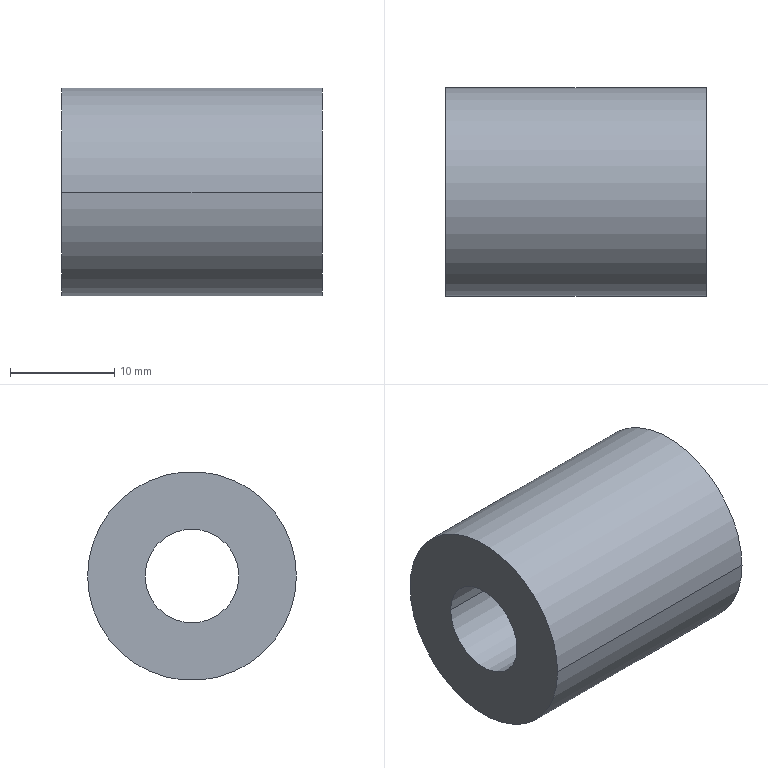Part | STEP file | LM-05-1262 | 1 solid | 6 faces | box 25 x 20 x 20 mm | volume 6264 mm3 | cylinder 4 | plane 2 | commonest cylinder face diameters 9 x2 20 x2
STEP:
#1=CARTESIAN_POINT('',(0.,0.,0.));
#2=DIRECTION('',(0.,0.,1.));
#3=DIRECTION('',(1.,0.,0.));
#4=AXIS2_PLACEMENT_3D('',#1,#2,#3);
#5=CARTESIAN_POINT('',(12.5,-4.5,0.));
#6=VERTEX_POINT('',#5);
#7=CARTESIAN_POINT('',(-12.5,-4.5,0.));
#8=VERTEX_POINT('',#7);
#9=CARTESIAN_POINT('',(12.5,-4.5,0.));
#10=DIRECTION('',(-1.,0.,0.));
#11=VECTOR('',#10,1.);
#12=LINE('',#9,#11);
#13=CARTESIAN_POINT('',(12.5,0.,0.));
#14=DIRECTION('',(-1.,0.,0.));
#15=DIRECTION('',(0.,-1.,0.));
#16=AXIS2_PLACEMENT_3D('',#13,#14,#15);
#17=CYLINDRICAL_SURFACE('',#16,4.5);
#18=CARTESIAN_POINT('',(6.283,0.));
#19=DIRECTION('',(0.,1.));
#20=VECTOR('',#19,1.);
#21=LINE('',#18,#20);
#22=(GEOMETRIC_REPRESENTATION_CONTEXT(2)PARAMETRIC_REPRESENTATION_CONTEXT()REPRESENTATION_CONTEXT('',''));
#23=DEFINITIONAL_REPRESENTATION('',(#21),#22);
#24=PCURVE('',#17,#23);
#25=CARTESIAN_POINT('',(12.5,0.,0.));
#26=DIRECTION('',(-1.,0.,0.));
#27=DIRECTION('',(0.,-1.,0.));
#28=AXIS2_PLACEMENT_3D('',#25,#26,#27);
#29=CYLINDRICAL_SURFACE('',#28,4.5);
#30=CARTESIAN_POINT('',(0.,0.));
#31=DIRECTION('',(0.,1.));
#32=VECTOR('',#31,1.);
#33=LINE('',#30,#32);
#34=(GEOMETRIC_REPRESENTATION_CONTEXT(2)PARAMETRIC_REPRESENTATION_CONTEXT()REPRESENTATION_CONTEXT('',''));
#35=DEFINITIONAL_REPRESENTATION('',(#33),#34);
#36=PCURVE('',#29,#35);
#37=SURFACE_CURVE('',#12,(#24,#36),.PCURVE_S1.);
#38=EDGE_CURVE('',#6,#8,#37,.T.);
#39=ORIENTED_EDGE('',*,*,#38,.T.);
#40=CARTESIAN_POINT('',(-12.5,4.5,0.));
#41=VERTEX_POINT('',#40);
#42=CARTESIAN_POINT('',(-12.5,0.,0.));
#43=DIRECTION('',(-1.,0.,0.));
#44=DIRECTION('',(0.,-1.,0.));
#45=AXIS2_PLACEMENT_3D('',#42,#43,#44);
#46=CIRCLE('',#45,4.5);
#47=CARTESIAN_POINT('',(0.,25.));
#48=DIRECTION('',(1.,0.));
#49=VECTOR('',#48,1.);
#50=LINE('',#47,#49);
#51=(GEOMETRIC_REPRESENTATION_CONTEXT(2)PARAMETRIC_REPRESENTATION_CONTEXT()REPRESENTATION_CONTEXT('',''));
#52=DEFINITIONAL_REPRESENTATION('',(#50),#51);
#53=PCURVE('',#17,#52);
#54=CARTESIAN_POINT('',(-12.5,4.5,0.));
#55=DIRECTION('',(-1.,0.,0.));
#56=DIRECTION('',(0.,-1.,0.));
#57=AXIS2_PLACEMENT_3D('',#54,#55,#56);
#58=PLANE('',#57);
#59=CARTESIAN_POINT('',(4.5,0.));
#60=DIRECTION('',(1.,0.));
#61=AXIS2_PLACEMENT_2D('',#59,#60);
#62=CIRCLE('',#61,4.5);
#63=(GEOMETRIC_REPRESENTATION_CONTEXT(2)PARAMETRIC_REPRESENTATION_CONTEXT()REPRESENTATION_CONTEXT('',''));
#64=DEFINITIONAL_REPRESENTATION('',(#62),#63);
#65=PCURVE('',#58,#64);
#66=SURFACE_CURVE('',#46,(#53,#65),.PCURVE_S1.);
#67=EDGE_CURVE('',#41,#8,#66,.T.);
#68=ORIENTED_EDGE('',*,*,#67,.F.);
#69=CARTESIAN_POINT('',(12.5,4.5,0.));
#70=VERTEX_POINT('',#69);
#71=CARTESIAN_POINT('',(12.5,4.5,0.));
#72=DIRECTION('',(-1.,0.,0.));
#73=VECTOR('',#72,1.);
#74=LINE('',#71,#73);
#75=CARTESIAN_POINT('',(3.142,0.));
#76=DIRECTION('',(0.,1.));
#77=VECTOR('',#76,1.);
#78=LINE('',#75,#77);
#79=(GEOMETRIC_REPRESENTATION_CONTEXT(2)PARAMETRIC_REPRESENTATION_CONTEXT()REPRESENTATION_CONTEXT('',''));
#80=DEFINITIONAL_REPRESENTATION('',(#78),#79);
#81=PCURVE('',#17,#80);
#82=CARTESIAN_POINT('',(3.142,0.));
#83=DIRECTION('',(0.,1.));
#84=VECTOR('',#83,1.);
#85=LINE('',#82,#84);
#86=(GEOMETRIC_REPRESENTATION_CONTEXT(2)PARAMETRIC_REPRESENTATION_CONTEXT()REPRESENTATION_CONTEXT('',''));
#87=DEFINITIONAL_REPRESENTATION('',(#85),#86);
#88=PCURVE('',#29,#87);
#89=SURFACE_CURVE('',#74,(#81,#88),.PCURVE_S1.);
#90=EDGE_CURVE('',#70,#41,#89,.T.);
#91=ORIENTED_EDGE('',*,*,#90,.F.);
#92=CARTESIAN_POINT('',(12.5,0.,0.));
#93=DIRECTION('',(-1.,0.,0.));
#94=DIRECTION('',(0.,-1.,0.));
#95=AXIS2_PLACEMENT_3D('',#92,#93,#94);
#96=CIRCLE('',#95,4.5);
#97=CARTESIAN_POINT('',(0.,0.));
#98=DIRECTION('',(1.,0.));
#99=VECTOR('',#98,1.);
#100=LINE('',#97,#99);
#101=(GEOMETRIC_REPRESENTATION_CONTEXT(2)PARAMETRIC_REPRESENTATION_CONTEXT()REPRESENTATION_CONTEXT('',''));
#102=DEFINITIONAL_REPRESENTATION('',(#100),#101);
#103=PCURVE('',#17,#102);
#104=CARTESIAN_POINT('',(12.5,10.,0.));
#105=DIRECTION('',(1.,0.,0.));
#106=DIRECTION('',(0.,1.,0.));
#107=AXIS2_PLACEMENT_3D('',#104,#105,#106);
#108=PLANE('',#107);
#109=CARTESIAN_POINT('',(-14.5,0.));
#110=CARTESIAN_POINT('',(-14.5,7.794));
#111=CARTESIAN_POINT('',(-7.75,3.897));
#112=CARTESIAN_POINT('',(-1.,0.));
#113=CARTESIAN_POINT('',(-7.75,-3.897));
#114=CARTESIAN_POINT('',(-14.5,-7.794));
#115=CARTESIAN_POINT('',(-14.5,0.));
#116=(BOUNDED_CURVE()B_SPLINE_CURVE(2,(#109,#110,#111,#112,#113,#114,#115),.UNSPECIFIED.,.T.,.F.)B_SPLINE_CURVE_WITH_KNOTS((1,2,2,2,2,1),(-2.094,0.,2.094,4.189,6.283,8.378),.UNSPECIFIED.)CURVE()GEOMETRIC_REPRESENTATION_ITEM()RATIONAL_B_SPLINE_CURVE((1.,0.5,1.,0.5,1.,0.5,1.))REPRESENTATION_ITEM(''));
#117=(GEOMETRIC_REPRESENTATION_CONTEXT(2)PARAMETRIC_REPRESENTATION_CONTEXT()REPRESENTATION_CONTEXT('',''));
#118=DEFINITIONAL_REPRESENTATION('',(#116),#117);
#119=PCURVE('',#108,#118);
#120=SURFACE_CURVE('',#96,(#103,#119),.PCURVE_S1.);
#121=EDGE_CURVE('',#70,#6,#120,.T.);
#122=ORIENTED_EDGE('',*,*,#121,.T.);
#123=EDGE_LOOP('',(#39,#68,#91,#122));
#124=FACE_BOUND('',#123,.F.);
#125=ADVANCED_FACE('',(#124),#17,.F.);
#126=CARTESIAN_POINT('',(12.5,-10.,0.));
#127=VERTEX_POINT('',#126);
#128=CARTESIAN_POINT('',(12.5,10.,0.));
#129=VERTEX_POINT('',#128);
#130=CARTESIAN_POINT('',(12.5,0.,0.));
#131=DIRECTION('',(-1.,0.,0.));
#132=DIRECTION('',(0.,-1.,0.));
#133=AXIS2_PLACEMENT_3D('',#130,#131,#132);
#134=CIRCLE('',#133,10.);
#135=CARTESIAN_POINT('',(12.5,0.,0.));
#136=DIRECTION('',(-1.,0.,0.));
#137=DIRECTION('',(0.,-1.,0.));
#138=AXIS2_PLACEMENT_3D('',#135,#136,#137);
#139=CYLINDRICAL_SURFACE('',#138,10.);
#140=CARTESIAN_POINT('',(0.,0.));
#141=DIRECTION('',(1.,0.));
#142=VECTOR('',#141,1.);
#143=LINE('',#140,#142);
#144=(GEOMETRIC_REPRESENTATION_CONTEXT(2)PARAMETRIC_REPRESENTATION_CONTEXT()REPRESENTATION_CONTEXT('',''));
#145=DEFINITIONAL_REPRESENTATION('',(#143),#144);
#146=PCURVE('',#139,#145);
#147=CARTESIAN_POINT('',(-20.,0.));
#148=CARTESIAN_POINT('',(-20.,17.321));
#149=CARTESIAN_POINT('',(-5.,8.66));
#150=CARTESIAN_POINT('',(10.,0.));
#151=CARTESIAN_POINT('',(-5.,-8.66));
#152=CARTESIAN_POINT('',(-20.,-17.321));
#153=CARTESIAN_POINT('',(-20.,0.));
#154=(BOUNDED_CURVE()B_SPLINE_CURVE(2,(#147,#148,#149,#150,#151,#152,#153),.UNSPECIFIED.,.T.,.F.)B_SPLINE_CURVE_WITH_KNOTS((1,2,2,2,2,1),(-2.094,0.,2.094,4.189,6.283,8.378),.UNSPECIFIED.)CURVE()GEOMETRIC_REPRESENTATION_ITEM()RATIONAL_B_SPLINE_CURVE((1.,0.5,1.,0.5,1.,0.5,1.))REPRESENTATION_ITEM(''));
#155=(GEOMETRIC_REPRESENTATION_CONTEXT(2)PARAMETRIC_REPRESENTATION_CONTEXT()REPRESENTATION_CONTEXT('',''));
#156=DEFINITIONAL_REPRESENTATION('',(#154),#155);
#157=PCURVE('',#108,#156);
#158=SURFACE_CURVE('',#134,(#146,#157),.PCURVE_S1.);
#159=EDGE_CURVE('',#127,#129,#158,.T.);
#160=ORIENTED_EDGE('',*,*,#159,.T.);
#161=CARTESIAN_POINT('',(-12.5,10.,0.));
#162=VERTEX_POINT('',#161);
#163=CARTESIAN_POINT('',(12.5,10.,0.));
#164=DIRECTION('',(-1.,0.,0.));
#165=VECTOR('',#164,1.);
#166=LINE('',#163,#165);
#167=CARTESIAN_POINT('',(3.142,0.));
#168=DIRECTION('',(0.,1.));
#169=VECTOR('',#168,1.);
#170=LINE('',#167,#169);
#171=(GEOMETRIC_REPRESENTATION_CONTEXT(2)PARAMETRIC_REPRESENTATION_CONTEXT()REPRESENTATION_CONTEXT('',''));
#172=DEFINITIONAL_REPRESENTATION('',(#170),#171);
#173=PCURVE('',#139,#172);
#174=CARTESIAN_POINT('',(12.5,0.,0.));
#175=DIRECTION('',(-1.,0.,0.));
#176=DIRECTION('',(0.,-1.,0.));
#177=AXIS2_PLACEMENT_3D('',#174,#175,#176);
#178=CYLINDRICAL_SURFACE('',#177,10.);
#179=CARTESIAN_POINT('',(3.142,0.));
#180=DIRECTION('',(0.,1.));
#181=VECTOR('',#180,1.);
#182=LINE('',#179,#181);
#183=(GEOMETRIC_REPRESENTATION_CONTEXT(2)PARAMETRIC_REPRESENTATION_CONTEXT()REPRESENTATION_CONTEXT('',''));
#184=DEFINITIONAL_REPRESENTATION('',(#182),#183);
#185=PCURVE('',#178,#184);
#186=SURFACE_CURVE('',#166,(#173,#185),.PCURVE_S1.);
#187=EDGE_CURVE('',#129,#162,#186,.T.);
#188=ORIENTED_EDGE('',*,*,#187,.T.);
#189=CARTESIAN_POINT('',(-12.5,-10.,0.));
#190=VERTEX_POINT('',#189);
#191=CARTESIAN_POINT('',(-12.5,0.,0.));
#192=DIRECTION('',(-1.,0.,0.));
#193=DIRECTION('',(0.,-1.,0.));
#194=AXIS2_PLACEMENT_3D('',#191,#192,#193);
#195=CIRCLE('',#194,10.);
#196=CARTESIAN_POINT('',(0.,25.));
#197=DIRECTION('',(1.,0.));
#198=VECTOR('',#197,1.);
#199=LINE('',#196,#198);
#200=(GEOMETRIC_REPRESENTATION_CONTEXT(2)PARAMETRIC_REPRESENTATION_CONTEXT()REPRESENTATION_CONTEXT('',''));
#201=DEFINITIONAL_REPRESENTATION('',(#199),#200);
#202=PCURVE('',#139,#201);
#203=CARTESIAN_POINT('',(4.5,0.));
#204=DIRECTION('',(1.,0.));
#205=AXIS2_PLACEMENT_2D('',#203,#204);
#206=CIRCLE('',#205,10.);
#207=(GEOMETRIC_REPRESENTATION_CONTEXT(2)PARAMETRIC_REPRESENTATION_CONTEXT()REPRESENTATION_CONTEXT('',''));
#208=DEFINITIONAL_REPRESENTATION('',(#206),#207);
#209=PCURVE('',#58,#208);
#210=SURFACE_CURVE('',#195,(#202,#209),.PCURVE_S1.);
#211=EDGE_CURVE('',#190,#162,#210,.T.);
#212=ORIENTED_EDGE('',*,*,#211,.F.);
#213=CARTESIAN_POINT('',(12.5,-10.,0.));
#214=DIRECTION('',(-1.,0.,0.));
#215=VECTOR('',#214,1.);
#216=LINE('',#213,#215);
#217=CARTESIAN_POINT('',(0.,0.));
#218=DIRECTION('',(0.,1.));
#219=VECTOR('',#218,1.);
#220=LINE('',#217,#219);
#221=(GEOMETRIC_REPRESENTATION_CONTEXT(2)PARAMETRIC_REPRESENTATION_CONTEXT()REPRESENTATION_CONTEXT('',''));
#222=DEFINITIONAL_REPRESENTATION('',(#220),#221);
#223=PCURVE('',#139,#222);
#224=CARTESIAN_POINT('',(6.283,0.));
#225=DIRECTION('',(0.,1.));
#226=VECTOR('',#225,1.);
#227=LINE('',#224,#226);
#228=(GEOMETRIC_REPRESENTATION_CONTEXT(2)PARAMETRIC_REPRESENTATION_CONTEXT()REPRESENTATION_CONTEXT('',''));
#229=DEFINITIONAL_REPRESENTATION('',(#227),#228);
#230=PCURVE('',#178,#229);
#231=SURFACE_CURVE('',#216,(#223,#230),.PCURVE_S1.);
#232=EDGE_CURVE('',#127,#190,#231,.T.);
#233=ORIENTED_EDGE('',*,*,#232,.F.);
#234=EDGE_LOOP('',(#160,#188,#212,#233));
#235=FACE_BOUND('',#234,.T.);
#236=ADVANCED_FACE('',(#235),#139,.T.);
#237=ORIENTED_EDGE('',*,*,#187,.F.);
#238=CARTESIAN_POINT('',(12.5,0.,0.));
#239=DIRECTION('',(-1.,0.,0.));
#240=DIRECTION('',(0.,-1.,0.));
#241=AXIS2_PLACEMENT_3D('',#238,#239,#240);
#242=CIRCLE('',#241,10.);
#243=CARTESIAN_POINT('',(0.,0.));
#244=DIRECTION('',(1.,0.));
#245=VECTOR('',#244,1.);
#246=LINE('',#243,#245);
#247=(GEOMETRIC_REPRESENTATION_CONTEXT(2)PARAMETRIC_REPRESENTATION_CONTEXT()REPRESENTATION_CONTEXT('',''));
#248=DEFINITIONAL_REPRESENTATION('',(#246),#247);
#249=PCURVE('',#178,#248);
#250=CARTESIAN_POINT('',(-20.,0.));
#251=CARTESIAN_POINT('',(-20.,17.321));
#252=CARTESIAN_POINT('',(-5.,8.66));
#253=CARTESIAN_POINT('',(10.,0.));
#254=CARTESIAN_POINT('',(-5.,-8.66));
#255=CARTESIAN_POINT('',(-20.,-17.321));
#256=CARTESIAN_POINT('',(-20.,0.));
#257=(BOUNDED_CURVE()B_SPLINE_CURVE(2,(#250,#251,#252,#253,#254,#255,#256),.UNSPECIFIED.,.T.,.F.)B_SPLINE_CURVE_WITH_KNOTS((1,2,2,2,2,1),(-2.094,0.,2.094,4.189,6.283,8.378),.UNSPECIFIED.)CURVE()GEOMETRIC_REPRESENTATION_ITEM()RATIONAL_B_SPLINE_CURVE((1.,0.5,1.,0.5,1.,0.5,1.))REPRESENTATION_ITEM(''));
#258=(GEOMETRIC_REPRESENTATION_CONTEXT(2)PARAMETRIC_REPRESENTATION_CONTEXT()REPRESENTATION_CONTEXT('',''));
#259=DEFINITIONAL_REPRESENTATION('',(#257),#258);
#260=PCURVE('',#108,#259);
#261=SURFACE_CURVE('',#242,(#249,#260),.PCURVE_S1.);
#262=EDGE_CURVE('',#129,#127,#261,.T.);
#263=ORIENTED_EDGE('',*,*,#262,.T.);
#264=ORIENTED_EDGE('',*,*,#232,.T.);
#265=CARTESIAN_POINT('',(-12.5,0.,0.));
#266=DIRECTION('',(-1.,0.,0.));
#267=DIRECTION('',(0.,-1.,0.));
#268=AXIS2_PLACEMENT_3D('',#265,#266,#267);
#269=CIRCLE('',#268,10.);
#270=CARTESIAN_POINT('',(0.,25.));
#271=DIRECTION('',(1.,0.));
#272=VECTOR('',#271,1.);
#273=LINE('',#270,#272);
#274=(GEOMETRIC_REPRESENTATION_CONTEXT(2)PARAMETRIC_REPRESENTATION_CONTEXT()REPRESENTATION_CONTEXT('',''));
#275=DEFINITIONAL_REPRESENTATION('',(#273),#274);
#276=PCURVE('',#178,#275);
#277=CARTESIAN_POINT('',(4.5,0.));
#278=DIRECTION('',(1.,0.));
#279=AXIS2_PLACEMENT_2D('',#277,#278);
#280=CIRCLE('',#279,10.);
#281=(GEOMETRIC_REPRESENTATION_CONTEXT(2)PARAMETRIC_REPRESENTATION_CONTEXT()REPRESENTATION_CONTEXT('',''));
#282=DEFINITIONAL_REPRESENTATION('',(#280),#281);
#283=PCURVE('',#58,#282);
#284=SURFACE_CURVE('',#269,(#276,#283),.PCURVE_S1.);
#285=EDGE_CURVE('',#162,#190,#284,.T.);
#286=ORIENTED_EDGE('',*,*,#285,.F.);
#287=EDGE_LOOP('',(#237,#263,#264,#286));
#288=FACE_BOUND('',#287,.T.);
#289=ADVANCED_FACE('',(#288),#178,.T.);
#290=CARTESIAN_POINT('',(12.5,0.,0.));
#291=DIRECTION('',(-1.,0.,0.));
#292=DIRECTION('',(0.,-1.,0.));
#293=AXIS2_PLACEMENT_3D('',#290,#291,#292);
#294=CIRCLE('',#293,4.5);
#295=CARTESIAN_POINT('',(-14.5,0.));
#296=CARTESIAN_POINT('',(-14.5,7.794));
#297=CARTESIAN_POINT('',(-7.75,3.897));
#298=CARTESIAN_POINT('',(-1.,0.));
#299=CARTESIAN_POINT('',(-7.75,-3.897));
#300=CARTESIAN_POINT('',(-14.5,-7.794));
#301=CARTESIAN_POINT('',(-14.5,0.));
#302=(BOUNDED_CURVE()B_SPLINE_CURVE(2,(#295,#296,#297,#298,#299,#300,#301),.UNSPECIFIED.,.T.,.F.)B_SPLINE_CURVE_WITH_KNOTS((1,2,2,2,2,1),(-2.094,0.,2.094,4.189,6.283,8.378),.UNSPECIFIED.)CURVE()GEOMETRIC_REPRESENTATION_ITEM()RATIONAL_B_SPLINE_CURVE((1.,0.5,1.,0.5,1.,0.5,1.))REPRESENTATION_ITEM(''));
#303=(GEOMETRIC_REPRESENTATION_CONTEXT(2)PARAMETRIC_REPRESENTATION_CONTEXT()REPRESENTATION_CONTEXT('',''));
#304=DEFINITIONAL_REPRESENTATION('',(#302),#303);
#305=PCURVE('',#108,#304);
#306=CARTESIAN_POINT('',(0.,0.));
#307=DIRECTION('',(1.,0.));
#308=VECTOR('',#307,1.);
#309=LINE('',#306,#308);
#310=(GEOMETRIC_REPRESENTATION_CONTEXT(2)PARAMETRIC_REPRESENTATION_CONTEXT()REPRESENTATION_CONTEXT('',''));
#311=DEFINITIONAL_REPRESENTATION('',(#309),#310);
#312=PCURVE('',#29,#311);
#313=SURFACE_CURVE('',#294,(#305,#312),.PCURVE_S1.);
#314=EDGE_CURVE('',#6,#70,#313,.T.);
#315=ORIENTED_EDGE('',*,*,#314,.T.);
#316=ORIENTED_EDGE('',*,*,#121,.T.);
#317=EDGE_LOOP('',(#315,#316));
#318=FACE_BOUND('',#317,.T.);
#319=ORIENTED_EDGE('',*,*,#159,.F.);
#320=ORIENTED_EDGE('',*,*,#262,.F.);
#321=EDGE_LOOP('',(#319,#320));
#322=FACE_BOUND('',#321,.T.);
#323=ADVANCED_FACE('',(#318,#322),#108,.T.);
#324=CARTESIAN_POINT('',(-12.5,0.,0.));
#325=DIRECTION('',(-1.,0.,0.));
#326=DIRECTION('',(0.,-1.,0.));
#327=AXIS2_PLACEMENT_3D('',#324,#325,#326);
#328=CIRCLE('',#327,4.5);
#329=CARTESIAN_POINT('',(0.,25.));
#330=DIRECTION('',(1.,0.));
#331=VECTOR('',#330,1.);
#332=LINE('',#329,#331);
#333=(GEOMETRIC_REPRESENTATION_CONTEXT(2)PARAMETRIC_REPRESENTATION_CONTEXT()REPRESENTATION_CONTEXT('',''));
#334=DEFINITIONAL_REPRESENTATION('',(#332),#333);
#335=PCURVE('',#29,#334);
#336=CARTESIAN_POINT('',(4.5,0.));
#337=DIRECTION('',(1.,0.));
#338=AXIS2_PLACEMENT_2D('',#336,#337);
#339=CIRCLE('',#338,4.5);
#340=(GEOMETRIC_REPRESENTATION_CONTEXT(2)PARAMETRIC_REPRESENTATION_CONTEXT()REPRESENTATION_CONTEXT('',''));
#341=DEFINITIONAL_REPRESENTATION('',(#339),#340);
#342=PCURVE('',#58,#341);
#343=SURFACE_CURVE('',#328,(#335,#342),.PCURVE_S1.);
#344=EDGE_CURVE('',#8,#41,#343,.T.);
#345=ORIENTED_EDGE('',*,*,#344,.F.);
#346=ORIENTED_EDGE('',*,*,#38,.F.);
#347=ORIENTED_EDGE('',*,*,#314,.T.);
#348=ORIENTED_EDGE('',*,*,#90,.T.);
#349=EDGE_LOOP('',(#345,#346,#347,#348));
#350=FACE_BOUND('',#349,.F.);
#351=ADVANCED_FACE('',(#350),#29,.F.);
#352=ORIENTED_EDGE('',*,*,#211,.T.);
#353=ORIENTED_EDGE('',*,*,#285,.T.);
#354=EDGE_LOOP('',(#352,#353));
#355=FACE_BOUND('',#354,.T.);
#356=ORIENTED_EDGE('',*,*,#344,.F.);
#357=ORIENTED_EDGE('',*,*,#67,.F.);
#358=EDGE_LOOP('',(#356,#357));
#359=FACE_BOUND('',#358,.T.);
#360=ADVANCED_FACE('',(#355,#359),#58,.T.);
#361=CLOSED_SHELL('',(#125,#236,#289,#323,#351,#360));
#362=MANIFOLD_SOLID_BREP('',#361);
#363=(LENGTH_UNIT()NAMED_UNIT(*)SI_UNIT(.MILLI.,.METRE.));
#364=UNCERTAINTY_MEASURE_WITH_UNIT(LENGTH_MEASURE(0.0000001),#363,'','');
#365=(NAMED_UNIT(*)PLANE_ANGLE_UNIT()SI_UNIT($,.RADIAN.));
#366=(NAMED_UNIT(*)SI_UNIT($,.STERADIAN.)SOLID_ANGLE_UNIT());
#367=(GEOMETRIC_REPRESENTATION_CONTEXT(3)GLOBAL_UNCERTAINTY_ASSIGNED_CONTEXT((#364))GLOBAL_UNIT_ASSIGNED_CONTEXT((#363,#365,#366))REPRESENTATION_CONTEXT('',''));
#368=ADVANCED_BREP_SHAPE_REPRESENTATION('',(#4,#362),#367);